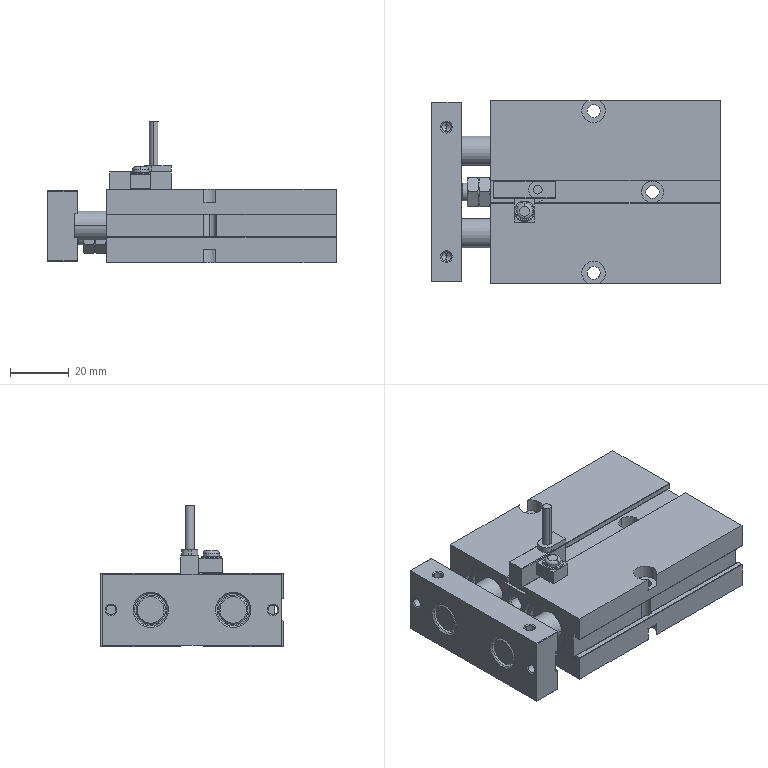Part | SolidWorks | 3 solids | 326 faces | box 98 x 62 x 48 mm | volume 117635 mm3 | plane 132 | cylinder 124 | cone 66 | torus 4 | commonest cylinder face diameters 0.4 x30 20 x16 3.242 x12 10 x12 4.5 x10 7.5 x8